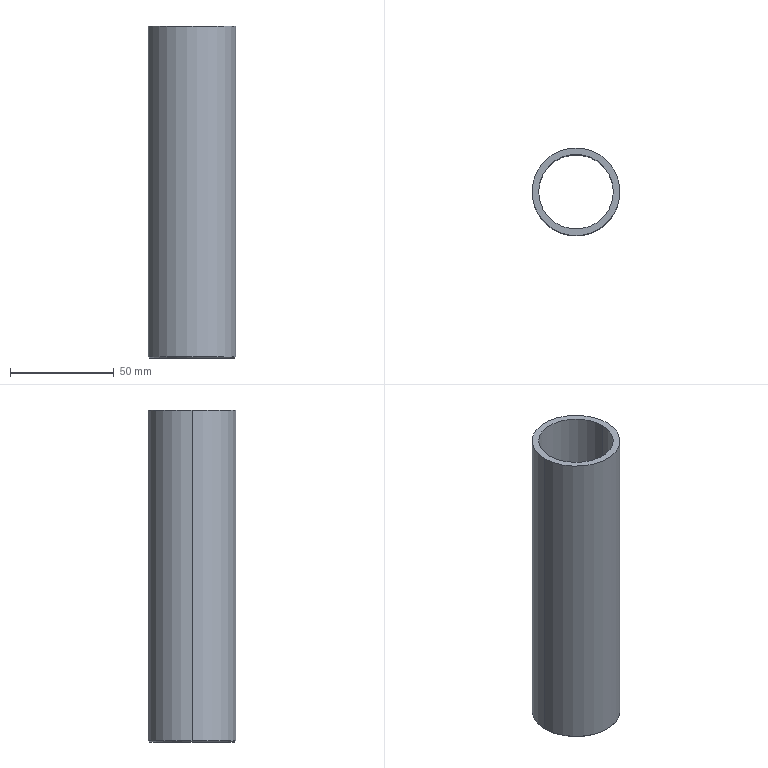Part | SolidWorks | features Chamfer 1, Extrusion 1, Shell 1 | 1 solid | 8 faces | box 42.4 x 42.4 x 160 mm | volume 63037 mm3 | cylinder 4 | cone 2 | plane 2 | commonest cylinder face diameters 36 x2 42.4 x2
STEP:
#1=CARTESIAN_POINT('',(-20.7,0.,0.));
#2=VERTEX_POINT('',#1);
#3=CARTESIAN_POINT('',(20.7,0.,0.));
#4=VERTEX_POINT('',#3);
#5=CARTESIAN_POINT('',(0.,0.,0.));
#6=DIRECTION('',(0.,0.,-1.));
#7=DIRECTION('',(1.,0.,0.));
#8=AXIS2_PLACEMENT_3D('',#5,#6,#7);
#9=CIRCLE('',#8,20.7);
#10=EDGE_CURVE('',#2,#4,#9,.T.);
#11=ORIENTED_EDGE('',*,*,#10,.F.);
#12=CARTESIAN_POINT('',(-21.2,0.,0.5));
#13=VERTEX_POINT('',#12);
#14=CARTESIAN_POINT('',(-21.2,0.,0.5));
#15=DIRECTION('',(-0.7071,0.,0.7071));
#16=VECTOR('',#15,1000.);
#17=LINE('',#14,#16);
#18=EDGE_CURVE('',#2,#13,#17,.T.);
#19=ORIENTED_EDGE('',*,*,#18,.T.);
#20=CARTESIAN_POINT('',(21.2,0.,0.5));
#21=VERTEX_POINT('',#20);
#22=CARTESIAN_POINT('',(0.,0.,0.5));
#23=DIRECTION('',(0.,0.,1.));
#24=DIRECTION('',(1.,0.,0.));
#25=AXIS2_PLACEMENT_3D('',#22,#23,#24);
#26=CIRCLE('',#25,21.2);
#27=EDGE_CURVE('',#21,#13,#26,.T.);
#28=ORIENTED_EDGE('',*,*,#27,.F.);
#29=CARTESIAN_POINT('',(21.2,0.,0.5));
#30=DIRECTION('',(0.7071,0.,0.7071));
#31=VECTOR('',#30,1000.);
#32=LINE('',#29,#31);
#33=EDGE_CURVE('',#4,#21,#32,.T.);
#34=ORIENTED_EDGE('',*,*,#33,.F.);
#35=EDGE_LOOP('',(#11,#19,#28,#34));
#36=FACE_OUTER_BOUND('',#35,.T.);
#37=CARTESIAN_POINT('',(0.,0.,0.5));
#38=DIRECTION('',(0.,0.,1.));
#39=DIRECTION('',(1.,0.,0.));
#40=AXIS2_PLACEMENT_3D('',#37,#38,#39);
#41=CONICAL_SURFACE('',#40,21.2,0.7854);
#42=ADVANCED_FACE('',(#36),#41,.T.);
#43=CARTESIAN_POINT('',(-18.,0.,160.));
#44=VERTEX_POINT('',#43);
#45=CARTESIAN_POINT('',(18.,0.,160.));
#46=VERTEX_POINT('',#45);
#47=CARTESIAN_POINT('',(0.,0.,160.));
#48=DIRECTION('',(0.,0.,1.));
#49=DIRECTION('',(1.,0.,0.));
#50=AXIS2_PLACEMENT_3D('',#47,#48,#49);
#51=CIRCLE('',#50,18.);
#52=EDGE_CURVE('',#44,#46,#51,.T.);
#53=ORIENTED_EDGE('',*,*,#52,.T.);
#54=CARTESIAN_POINT('',(18.,0.,0.));
#55=VERTEX_POINT('',#54);
#56=CARTESIAN_POINT('',(18.,0.,160.));
#57=DIRECTION('',(0.,0.,-1.));
#58=VECTOR('',#57,1000.);
#59=LINE('',#56,#58);
#60=EDGE_CURVE('',#46,#55,#59,.T.);
#61=ORIENTED_EDGE('',*,*,#60,.T.);
#62=CARTESIAN_POINT('',(-18.,0.,0.));
#63=VERTEX_POINT('',#62);
#64=CARTESIAN_POINT('',(0.,0.,0.));
#65=DIRECTION('',(0.,0.,1.));
#66=DIRECTION('',(1.,0.,0.));
#67=AXIS2_PLACEMENT_3D('',#64,#65,#66);
#68=CIRCLE('',#67,18.);
#69=EDGE_CURVE('',#63,#55,#68,.T.);
#70=ORIENTED_EDGE('',*,*,#69,.F.);
#71=CARTESIAN_POINT('',(-18.,0.,160.));
#72=DIRECTION('',(0.,0.,-1.));
#73=VECTOR('',#72,1000.);
#74=LINE('',#71,#73);
#75=EDGE_CURVE('',#44,#63,#74,.T.);
#76=ORIENTED_EDGE('',*,*,#75,.F.);
#77=EDGE_LOOP('',(#53,#61,#70,#76));
#78=FACE_OUTER_BOUND('',#77,.T.);
#79=CARTESIAN_POINT('',(0.,0.,160.));
#80=DIRECTION('',(0.,0.,-1.));
#81=DIRECTION('',(-1.,0.,0.));
#82=AXIS2_PLACEMENT_3D('',#79,#80,#81);
#83=CYLINDRICAL_SURFACE('',#82,18.);
#84=ADVANCED_FACE('',(#78),#83,.F.);
#85=CARTESIAN_POINT('',(21.2,0.,160.));
#86=VERTEX_POINT('',#85);
#87=CARTESIAN_POINT('',(-21.2,0.,160.));
#88=VERTEX_POINT('',#87);
#89=CARTESIAN_POINT('',(0.,0.,160.));
#90=DIRECTION('',(0.,0.,1.));
#91=DIRECTION('',(1.,0.,0.));
#92=AXIS2_PLACEMENT_3D('',#89,#90,#91);
#93=CIRCLE('',#92,21.2);
#94=EDGE_CURVE('',#86,#88,#93,.T.);
#95=ORIENTED_EDGE('',*,*,#94,.F.);
#96=CARTESIAN_POINT('',(21.2,0.,160.));
#97=DIRECTION('',(0.,0.,-1.));
#98=VECTOR('',#97,1000.);
#99=LINE('',#96,#98);
#100=EDGE_CURVE('',#86,#21,#99,.T.);
#101=ORIENTED_EDGE('',*,*,#100,.T.);
#102=ORIENTED_EDGE('',*,*,#27,.T.);
#103=CARTESIAN_POINT('',(-21.2,0.,160.));
#104=DIRECTION('',(0.,0.,-1.));
#105=VECTOR('',#104,1000.);
#106=LINE('',#103,#105);
#107=EDGE_CURVE('',#88,#13,#106,.T.);
#108=ORIENTED_EDGE('',*,*,#107,.F.);
#109=EDGE_LOOP('',(#95,#101,#102,#108));
#110=FACE_OUTER_BOUND('',#109,.T.);
#111=CARTESIAN_POINT('',(0.,0.,160.));
#112=DIRECTION('',(0.,0.,-1.));
#113=DIRECTION('',(-1.,0.,0.));
#114=AXIS2_PLACEMENT_3D('',#111,#112,#113);
#115=CYLINDRICAL_SURFACE('',#114,21.2);
#116=ADVANCED_FACE('',(#110),#115,.T.);
#117=ORIENTED_EDGE('',*,*,#100,.F.);
#118=CARTESIAN_POINT('',(0.,0.,160.));
#119=DIRECTION('',(0.,0.,1.));
#120=DIRECTION('',(1.,0.,0.));
#121=AXIS2_PLACEMENT_3D('',#118,#119,#120);
#122=CIRCLE('',#121,21.2);
#123=EDGE_CURVE('',#88,#86,#122,.T.);
#124=ORIENTED_EDGE('',*,*,#123,.F.);
#125=ORIENTED_EDGE('',*,*,#107,.T.);
#126=CARTESIAN_POINT('',(0.,0.,0.5));
#127=DIRECTION('',(0.,0.,1.));
#128=DIRECTION('',(1.,0.,0.));
#129=AXIS2_PLACEMENT_3D('',#126,#127,#128);
#130=CIRCLE('',#129,21.2);
#131=EDGE_CURVE('',#13,#21,#130,.T.);
#132=ORIENTED_EDGE('',*,*,#131,.T.);
#133=EDGE_LOOP('',(#117,#124,#125,#132));
#134=FACE_OUTER_BOUND('',#133,.T.);
#135=CARTESIAN_POINT('',(0.,0.,160.));
#136=DIRECTION('',(0.,0.,-1.));
#137=DIRECTION('',(-1.,0.,0.));
#138=AXIS2_PLACEMENT_3D('',#135,#136,#137);
#139=CYLINDRICAL_SURFACE('',#138,21.2);
#140=ADVANCED_FACE('',(#134),#139,.T.);
#141=ORIENTED_EDGE('',*,*,#52,.F.);
#142=CARTESIAN_POINT('',(0.,0.,160.));
#143=DIRECTION('',(0.,0.,1.));
#144=DIRECTION('',(1.,0.,0.));
#145=AXIS2_PLACEMENT_3D('',#142,#143,#144);
#146=CIRCLE('',#145,18.);
#147=EDGE_CURVE('',#46,#44,#146,.T.);
#148=ORIENTED_EDGE('',*,*,#147,.F.);
#149=EDGE_LOOP('',(#141,#148));
#150=FACE_BOUND('',#149,.T.);
#151=ORIENTED_EDGE('',*,*,#123,.T.);
#152=ORIENTED_EDGE('',*,*,#94,.T.);
#153=EDGE_LOOP('',(#151,#152));
#154=FACE_OUTER_BOUND('',#153,.T.);
#155=CARTESIAN_POINT('',(0.,0.,160.));
#156=DIRECTION('',(0.,0.,1.));
#157=DIRECTION('',(1.,0.,0.));
#158=AXIS2_PLACEMENT_3D('',#155,#156,#157);
#159=PLANE('',#158);
#160=ADVANCED_FACE('',(#150,#154),#159,.T.);
#161=CARTESIAN_POINT('',(0.,0.,0.));
#162=DIRECTION('',(0.,0.,-1.));
#163=DIRECTION('',(1.,0.,0.));
#164=AXIS2_PLACEMENT_3D('',#161,#162,#163);
#165=CIRCLE('',#164,20.7);
#166=EDGE_CURVE('',#4,#2,#165,.T.);
#167=ORIENTED_EDGE('',*,*,#166,.T.);
#168=ORIENTED_EDGE('',*,*,#10,.T.);
#169=EDGE_LOOP('',(#167,#168));
#170=FACE_OUTER_BOUND('',#169,.T.);
#171=ORIENTED_EDGE('',*,*,#69,.T.);
#172=CARTESIAN_POINT('',(0.,0.,0.));
#173=DIRECTION('',(0.,0.,1.));
#174=DIRECTION('',(1.,0.,0.));
#175=AXIS2_PLACEMENT_3D('',#172,#173,#174);
#176=CIRCLE('',#175,18.);
#177=EDGE_CURVE('',#55,#63,#176,.T.);
#178=ORIENTED_EDGE('',*,*,#177,.T.);
#179=EDGE_LOOP('',(#171,#178));
#180=FACE_BOUND('',#179,.T.);
#181=CARTESIAN_POINT('',(0.,0.,0.));
#182=DIRECTION('',(0.,0.,1.));
#183=DIRECTION('',(1.,0.,0.));
#184=AXIS2_PLACEMENT_3D('',#181,#182,#183);
#185=PLANE('',#184);
#186=ADVANCED_FACE('',(#170,#180),#185,.F.);
#187=ORIENTED_EDGE('',*,*,#60,.F.);
#188=ORIENTED_EDGE('',*,*,#147,.T.);
#189=ORIENTED_EDGE('',*,*,#75,.T.);
#190=ORIENTED_EDGE('',*,*,#177,.F.);
#191=EDGE_LOOP('',(#187,#188,#189,#190));
#192=FACE_OUTER_BOUND('',#191,.T.);
#193=CARTESIAN_POINT('',(0.,0.,160.));
#194=DIRECTION('',(0.,0.,-1.));
#195=DIRECTION('',(-1.,0.,0.));
#196=AXIS2_PLACEMENT_3D('',#193,#194,#195);
#197=CYLINDRICAL_SURFACE('',#196,18.);
#198=ADVANCED_FACE('',(#192),#197,.F.);
#199=ORIENTED_EDGE('',*,*,#18,.F.);
#200=ORIENTED_EDGE('',*,*,#166,.F.);
#201=ORIENTED_EDGE('',*,*,#33,.T.);
#202=ORIENTED_EDGE('',*,*,#131,.F.);
#203=EDGE_LOOP('',(#199,#200,#201,#202));
#204=FACE_OUTER_BOUND('',#203,.T.);
#205=CARTESIAN_POINT('',(0.,0.,0.5));
#206=DIRECTION('',(0.,0.,1.));
#207=DIRECTION('',(1.,0.,0.));
#208=AXIS2_PLACEMENT_3D('',#205,#206,#207);
#209=CONICAL_SURFACE('',#208,21.2,0.7854);
#210=ADVANCED_FACE('',(#204),#209,.T.);
#211=CLOSED_SHELL('',(#42,#84,#116,#140,#160,#186,#198,#210));
#212=MANIFOLD_SOLID_BREP('',#211);
#213=CARTESIAN_POINT('',(0.,0.,0.));
#214=DIRECTION('',(0.,0.,1.));
#215=DIRECTION('',(1.,0.,0.));
#216=AXIS2_PLACEMENT_3D('',#213,#214,#215);
#217=(LENGTH_UNIT()NAMED_UNIT(*)SI_UNIT(.MILLI.,.METRE.));
#218=UNCERTAINTY_MEASURE_WITH_UNIT(LENGTH_MEASURE(0.00001),#217,'','');
#219=(NAMED_UNIT(*)PLANE_ANGLE_UNIT()SI_UNIT($,.RADIAN.));
#220=(NAMED_UNIT(*)SI_UNIT($,.STERADIAN.)SOLID_ANGLE_UNIT());
#221=(GEOMETRIC_REPRESENTATION_CONTEXT(3)GLOBAL_UNCERTAINTY_ASSIGNED_CONTEXT((#218))GLOBAL_UNIT_ASSIGNED_CONTEXT((#217,#219,#220))REPRESENTATION_CONTEXT('',''));
#222=ADVANCED_BREP_SHAPE_REPRESENTATION('',(#212,#216),#221);